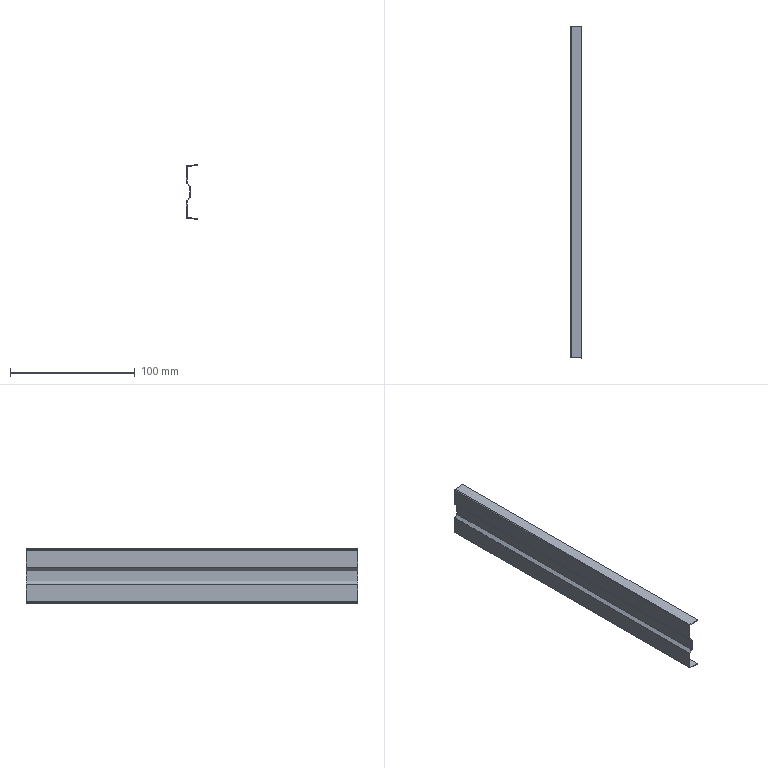Part | NX | features RETAINER-1_5003_009_C-SRH51Y22 2 | 1 solid | 24 faces | box 8.852 x 266.1 x 43.74 mm | volume 9676 mm3 | plane 18 | cylinder 6 | commonest cylinder face diameters 0.8 x4 1.2 x2
STEP:
#1=CARTESIAN_POINT('',(-207.227,-97.3,-65.352));
#2=VERTEX_POINT('',#1);
#3=CARTESIAN_POINT('',(-198.975,-97.3,-64.63));
#4=VERTEX_POINT('',#3);
#5=CARTESIAN_POINT('',(-207.775,-97.3,-65.4));
#6=DIRECTION('',(0.9962,0.,0.08716));
#7=VECTOR('',#6,1000.);
#8=LINE('',#5,#7);
#9=EDGE_CURVE('',#2,#4,#8,.T.);
#10=ORIENTED_EDGE('',*,*,#9,.F.);
#11=CARTESIAN_POINT('',(-207.227,-363.4,-65.352));
#12=VERTEX_POINT('',#11);
#13=CARTESIAN_POINT('',(-207.227,-97.3,-65.352));
#14=DIRECTION('',(0.,-1.,0.));
#15=VECTOR('',#14,1000.);
#16=LINE('',#13,#15);
#17=EDGE_CURVE('',#2,#12,#16,.T.);
#18=ORIENTED_EDGE('',*,*,#17,.T.);
#19=CARTESIAN_POINT('',(-198.975,-363.4,-64.63));
#20=VERTEX_POINT('',#19);
#21=CARTESIAN_POINT('',(-207.775,-363.4,-65.4));
#22=DIRECTION('',(0.9962,0.,0.08716));
#23=VECTOR('',#22,1000.);
#24=LINE('',#21,#23);
#25=EDGE_CURVE('',#12,#20,#24,.T.);
#26=ORIENTED_EDGE('',*,*,#25,.T.);
#27=CARTESIAN_POINT('',(-198.975,-97.3,-64.63));
#28=DIRECTION('',(0.,-1.,0.));
#29=VECTOR('',#28,1000.);
#30=LINE('',#27,#29);
#31=EDGE_CURVE('',#4,#20,#30,.T.);
#32=ORIENTED_EDGE('',*,*,#31,.F.);
#33=EDGE_LOOP('',(#10,#18,#26,#32));
#34=FACE_BOUND('',#33,.T.);
#35=CARTESIAN_POINT('',(-207.775,-97.3,-65.4));
#36=DIRECTION('',(0.08716,0.,-0.9962));
#37=DIRECTION('',(-0.9962,0.,-0.08716));
#38=AXIS2_PLACEMENT_3D('',#35,#36,#37);
#39=PLANE('',#38);
#40=ADVANCED_FACE('',(#34),#39,.F.);
#41=CARTESIAN_POINT('',(-198.923,-363.4,-65.228));
#42=VERTEX_POINT('',#41);
#43=CARTESIAN_POINT('',(-198.975,-363.4,-64.63));
#44=DIRECTION('',(0.08716,0.,-0.9962));
#45=VECTOR('',#44,1000.);
#46=LINE('',#43,#45);
#47=EDGE_CURVE('',#20,#42,#46,.T.);
#48=ORIENTED_EDGE('',*,*,#47,.T.);
#49=CARTESIAN_POINT('',(-198.923,-97.3,-65.228));
#50=VERTEX_POINT('',#49);
#51=CARTESIAN_POINT('',(-198.923,-97.3,-65.228));
#52=DIRECTION('',(0.,-1.,0.));
#53=VECTOR('',#52,1000.);
#54=LINE('',#51,#53);
#55=EDGE_CURVE('',#50,#42,#54,.T.);
#56=ORIENTED_EDGE('',*,*,#55,.F.);
#57=CARTESIAN_POINT('',(-198.975,-97.3,-64.63));
#58=DIRECTION('',(0.08716,0.,-0.9962));
#59=VECTOR('',#58,1000.);
#60=LINE('',#57,#59);
#61=EDGE_CURVE('',#4,#50,#60,.T.);
#62=ORIENTED_EDGE('',*,*,#61,.F.);
#63=ORIENTED_EDGE('',*,*,#31,.T.);
#64=EDGE_LOOP('',(#48,#56,#62,#63));
#65=FACE_BOUND('',#64,.T.);
#66=CARTESIAN_POINT('',(-198.975,-97.3,-64.63));
#67=DIRECTION('',(-0.9962,0.,-0.08716));
#68=DIRECTION('',(-0.08716,0.,0.9962));
#69=AXIS2_PLACEMENT_3D('',#66,#67,#68);
#70=PLANE('',#69);
#71=ADVANCED_FACE('',(#65),#70,.F.);
#72=CARTESIAN_POINT('',(-207.175,-363.4,-65.95));
#73=VERTEX_POINT('',#72);
#74=CARTESIAN_POINT('',(-207.175,-363.4,-65.95));
#75=DIRECTION('',(-0.9962,0.,-0.08716));
#76=VECTOR('',#75,1000.);
#77=LINE('',#74,#76);
#78=EDGE_CURVE('',#42,#73,#77,.T.);
#79=ORIENTED_EDGE('',*,*,#78,.T.);
#80=CARTESIAN_POINT('',(-207.175,-97.3,-65.95));
#81=VERTEX_POINT('',#80);
#82=CARTESIAN_POINT('',(-207.175,-97.3,-65.95));
#83=DIRECTION('',(0.,-1.,0.));
#84=VECTOR('',#83,1000.);
#85=LINE('',#82,#84);
#86=EDGE_CURVE('',#81,#73,#85,.T.);
#87=ORIENTED_EDGE('',*,*,#86,.F.);
#88=CARTESIAN_POINT('',(-207.175,-97.3,-65.95));
#89=DIRECTION('',(-0.9962,0.,-0.08716));
#90=VECTOR('',#89,1000.);
#91=LINE('',#88,#90);
#92=EDGE_CURVE('',#50,#81,#91,.T.);
#93=ORIENTED_EDGE('',*,*,#92,.F.);
#94=ORIENTED_EDGE('',*,*,#55,.T.);
#95=EDGE_LOOP('',(#79,#87,#93,#94));
#96=FACE_BOUND('',#95,.T.);
#97=CARTESIAN_POINT('',(-207.175,-97.3,-65.95));
#98=DIRECTION('',(-0.08716,0.,0.9962));
#99=DIRECTION('',(0.9962,0.,0.08716));
#100=AXIS2_PLACEMENT_3D('',#97,#98,#99);
#101=PLANE('',#100);
#102=ADVANCED_FACE('',(#96),#101,.F.);
#103=CARTESIAN_POINT('',(-207.175,-363.4,-79.4));
#104=VERTEX_POINT('',#103);
#105=CARTESIAN_POINT('',(-207.175,-363.4,-65.95));
#106=DIRECTION('',(0.,0.,-1.));
#107=VECTOR('',#106,1000.);
#108=LINE('',#105,#107);
#109=EDGE_CURVE('',#73,#104,#108,.T.);
#110=ORIENTED_EDGE('',*,*,#109,.T.);
#111=CARTESIAN_POINT('',(-207.175,-97.3,-79.4));
#112=VERTEX_POINT('',#111);
#113=CARTESIAN_POINT('',(-207.175,-97.3,-79.4));
#114=DIRECTION('',(0.,-1.,0.));
#115=VECTOR('',#114,1000.);
#116=LINE('',#113,#115);
#117=EDGE_CURVE('',#112,#104,#116,.T.);
#118=ORIENTED_EDGE('',*,*,#117,.F.);
#119=CARTESIAN_POINT('',(-207.175,-97.3,-65.95));
#120=DIRECTION('',(0.,0.,-1.));
#121=VECTOR('',#120,1000.);
#122=LINE('',#119,#121);
#123=EDGE_CURVE('',#81,#112,#122,.T.);
#124=ORIENTED_EDGE('',*,*,#123,.F.);
#125=ORIENTED_EDGE('',*,*,#86,.T.);
#126=EDGE_LOOP('',(#110,#118,#124,#125));
#127=FACE_BOUND('',#126,.T.);
#128=CARTESIAN_POINT('',(-207.175,-97.3,-65.95));
#129=DIRECTION('',(-1.,0.,0.));
#130=DIRECTION('',(0.,-1.,0.));
#131=AXIS2_PLACEMENT_3D('',#128,#129,#130);
#132=PLANE('',#131);
#133=ADVANCED_FACE('',(#127),#132,.F.);
#134=CARTESIAN_POINT('',(-204.792,-363.4,-81.783));
#135=VERTEX_POINT('',#134);
#136=CARTESIAN_POINT('',(-204.675,-363.4,-81.9));
#137=DIRECTION('',(0.7071,0.,-0.7071));
#138=VECTOR('',#137,1000.);
#139=LINE('',#136,#138);
#140=EDGE_CURVE('',#104,#135,#139,.T.);
#141=ORIENTED_EDGE('',*,*,#140,.T.);
#142=CARTESIAN_POINT('',(-204.792,-97.3,-81.783));
#143=VERTEX_POINT('',#142);
#144=CARTESIAN_POINT('',(-204.792,-97.3,-81.783));
#145=DIRECTION('',(0.,-1.,0.));
#146=VECTOR('',#145,1000.);
#147=LINE('',#144,#146);
#148=EDGE_CURVE('',#135,#143,#147,.F.);
#149=ORIENTED_EDGE('',*,*,#148,.T.);
#150=CARTESIAN_POINT('',(-204.675,-97.3,-81.9));
#151=DIRECTION('',(0.7071,0.,-0.7071));
#152=VECTOR('',#151,1000.);
#153=LINE('',#150,#152);
#154=EDGE_CURVE('',#112,#143,#153,.T.);
#155=ORIENTED_EDGE('',*,*,#154,.F.);
#156=ORIENTED_EDGE('',*,*,#117,.T.);
#157=EDGE_LOOP('',(#141,#149,#155,#156));
#158=FACE_BOUND('',#157,.T.);
#159=CARTESIAN_POINT('',(-204.675,-97.3,-81.9));
#160=DIRECTION('',(-0.7071,0.,-0.7071));
#161=DIRECTION('',(-0.7071,0.,0.7071));
#162=AXIS2_PLACEMENT_3D('',#159,#160,#161);
#163=PLANE('',#162);
#164=ADVANCED_FACE('',(#158),#163,.F.);
#165=CARTESIAN_POINT('',(-204.675,-363.4,-82.066));
#166=VERTEX_POINT('',#165);
#167=CARTESIAN_POINT('',(-204.675,-363.4,-90.934));
#168=VERTEX_POINT('',#167);
#169=CARTESIAN_POINT('',(-204.675,-363.4,-91.1));
#170=DIRECTION('',(0.,0.,-1.));
#171=VECTOR('',#170,1000.);
#172=LINE('',#169,#171);
#173=EDGE_CURVE('',#166,#168,#172,.T.);
#174=ORIENTED_EDGE('',*,*,#173,.T.);
#175=CARTESIAN_POINT('',(-204.675,-97.3,-90.934));
#176=VERTEX_POINT('',#175);
#177=CARTESIAN_POINT('',(-204.675,-97.3,-90.934));
#178=DIRECTION('',(0.,-1.,0.));
#179=VECTOR('',#178,1000.);
#180=LINE('',#177,#179);
#181=EDGE_CURVE('',#168,#176,#180,.F.);
#182=ORIENTED_EDGE('',*,*,#181,.T.);
#183=CARTESIAN_POINT('',(-204.675,-97.3,-82.066));
#184=VERTEX_POINT('',#183);
#185=CARTESIAN_POINT('',(-204.675,-97.3,-91.1));
#186=DIRECTION('',(0.,0.,-1.));
#187=VECTOR('',#186,1000.);
#188=LINE('',#185,#187);
#189=EDGE_CURVE('',#184,#176,#188,.T.);
#190=ORIENTED_EDGE('',*,*,#189,.F.);
#191=CARTESIAN_POINT('',(-204.675,-97.3,-82.066));
#192=DIRECTION('',(0.,-1.,0.));
#193=VECTOR('',#192,1000.);
#194=LINE('',#191,#193);
#195=EDGE_CURVE('',#184,#166,#194,.T.);
#196=ORIENTED_EDGE('',*,*,#195,.T.);
#197=EDGE_LOOP('',(#174,#182,#190,#196));
#198=FACE_BOUND('',#197,.T.);
#199=CARTESIAN_POINT('',(-204.675,-97.3,-91.1));
#200=DIRECTION('',(-1.,0.,0.));
#201=DIRECTION('',(0.,-1.,0.));
#202=AXIS2_PLACEMENT_3D('',#199,#200,#201);
#203=PLANE('',#202);
#204=ADVANCED_FACE('',(#198),#203,.F.);
#205=CARTESIAN_POINT('',(-204.792,-97.3,-91.217));
#206=VERTEX_POINT('',#205);
#207=CARTESIAN_POINT('',(-207.175,-97.3,-93.6));
#208=VERTEX_POINT('',#207);
#209=CARTESIAN_POINT('',(-204.675,-97.3,-91.1));
#210=DIRECTION('',(-0.7071,0.,-0.7071));
#211=VECTOR('',#210,1000.);
#212=LINE('',#209,#211);
#213=EDGE_CURVE('',#206,#208,#212,.T.);
#214=ORIENTED_EDGE('',*,*,#213,.F.);
#215=CARTESIAN_POINT('',(-204.792,-363.4,-91.217));
#216=VERTEX_POINT('',#215);
#217=CARTESIAN_POINT('',(-204.792,-97.3,-91.217));
#218=DIRECTION('',(0.,-1.,0.));
#219=VECTOR('',#218,1000.);
#220=LINE('',#217,#219);
#221=EDGE_CURVE('',#206,#216,#220,.T.);
#222=ORIENTED_EDGE('',*,*,#221,.T.);
#223=CARTESIAN_POINT('',(-207.175,-363.4,-93.6));
#224=VERTEX_POINT('',#223);
#225=CARTESIAN_POINT('',(-204.675,-363.4,-91.1));
#226=DIRECTION('',(-0.7071,0.,-0.7071));
#227=VECTOR('',#226,1000.);
#228=LINE('',#225,#227);
#229=EDGE_CURVE('',#216,#224,#228,.T.);
#230=ORIENTED_EDGE('',*,*,#229,.T.);
#231=CARTESIAN_POINT('',(-207.175,-97.3,-93.6));
#232=DIRECTION('',(0.,-1.,0.));
#233=VECTOR('',#232,1000.);
#234=LINE('',#231,#233);
#235=EDGE_CURVE('',#208,#224,#234,.T.);
#236=ORIENTED_EDGE('',*,*,#235,.F.);
#237=EDGE_LOOP('',(#214,#222,#230,#236));
#238=FACE_BOUND('',#237,.T.);
#239=CARTESIAN_POINT('',(-204.675,-97.3,-91.1));
#240=DIRECTION('',(-0.7071,0.,0.7071));
#241=DIRECTION('',(0.7071,0.,0.7071));
#242=AXIS2_PLACEMENT_3D('',#239,#240,#241);
#243=PLANE('',#242);
#244=ADVANCED_FACE('',(#238),#243,.F.);
#245=CARTESIAN_POINT('',(-207.175,-363.4,-107.05));
#246=VERTEX_POINT('',#245);
#247=CARTESIAN_POINT('',(-207.175,-363.4,-107.05));
#248=DIRECTION('',(0.,0.,-1.));
#249=VECTOR('',#248,1000.);
#250=LINE('',#247,#249);
#251=EDGE_CURVE('',#224,#246,#250,.T.);
#252=ORIENTED_EDGE('',*,*,#251,.T.);
#253=CARTESIAN_POINT('',(-207.175,-97.3,-107.05));
#254=VERTEX_POINT('',#253);
#255=CARTESIAN_POINT('',(-207.175,-97.3,-107.05));
#256=DIRECTION('',(0.,-1.,0.));
#257=VECTOR('',#256,1000.);
#258=LINE('',#255,#257);
#259=EDGE_CURVE('',#254,#246,#258,.T.);
#260=ORIENTED_EDGE('',*,*,#259,.F.);
#261=CARTESIAN_POINT('',(-207.175,-97.3,-107.05));
#262=DIRECTION('',(0.,0.,-1.));
#263=VECTOR('',#262,1000.);
#264=LINE('',#261,#263);
#265=EDGE_CURVE('',#208,#254,#264,.T.);
#266=ORIENTED_EDGE('',*,*,#265,.F.);
#267=ORIENTED_EDGE('',*,*,#235,.T.);
#268=EDGE_LOOP('',(#252,#260,#266,#267));
#269=FACE_BOUND('',#268,.T.);
#270=CARTESIAN_POINT('',(-207.175,-97.3,-107.05));
#271=DIRECTION('',(-1.,0.,0.));
#272=DIRECTION('',(0.,-1.,0.));
#273=AXIS2_PLACEMENT_3D('',#270,#271,#272);
#274=PLANE('',#273);
#275=ADVANCED_FACE('',(#269),#274,.F.);
#276=CARTESIAN_POINT('',(-198.923,-363.4,-107.772));
#277=VERTEX_POINT('',#276);
#278=CARTESIAN_POINT('',(-207.175,-363.4,-107.05));
#279=DIRECTION('',(0.9962,0.,-0.08716));
#280=VECTOR('',#279,1000.);
#281=LINE('',#278,#280);
#282=EDGE_CURVE('',#246,#277,#281,.T.);
#283=ORIENTED_EDGE('',*,*,#282,.T.);
#284=CARTESIAN_POINT('',(-198.923,-97.3,-107.772));
#285=VERTEX_POINT('',#284);
#286=CARTESIAN_POINT('',(-198.923,-97.3,-107.772));
#287=DIRECTION('',(0.,-1.,0.));
#288=VECTOR('',#287,1000.);
#289=LINE('',#286,#288);
#290=EDGE_CURVE('',#285,#277,#289,.T.);
#291=ORIENTED_EDGE('',*,*,#290,.F.);
#292=CARTESIAN_POINT('',(-207.175,-97.3,-107.05));
#293=DIRECTION('',(0.9962,0.,-0.08716));
#294=VECTOR('',#293,1000.);
#295=LINE('',#292,#294);
#296=EDGE_CURVE('',#254,#285,#295,.T.);
#297=ORIENTED_EDGE('',*,*,#296,.F.);
#298=ORIENTED_EDGE('',*,*,#259,.T.);
#299=EDGE_LOOP('',(#283,#291,#297,#298));
#300=FACE_BOUND('',#299,.T.);
#301=CARTESIAN_POINT('',(-207.175,-97.3,-107.05));
#302=DIRECTION('',(-0.08716,0.,-0.9962));
#303=DIRECTION('',(-0.9962,0.,0.08716));
#304=AXIS2_PLACEMENT_3D('',#301,#302,#303);
#305=PLANE('',#304);
#306=ADVANCED_FACE('',(#300),#305,.F.);
#307=CARTESIAN_POINT('',(-198.975,-363.4,-108.37));
#308=VERTEX_POINT('',#307);
#309=CARTESIAN_POINT('',(-198.923,-363.4,-107.772));
#310=DIRECTION('',(-0.08716,0.,-0.9962));
#311=VECTOR('',#310,1000.);
#312=LINE('',#309,#311);
#313=EDGE_CURVE('',#277,#308,#312,.T.);
#314=ORIENTED_EDGE('',*,*,#313,.T.);
#315=CARTESIAN_POINT('',(-198.975,-97.3,-108.37));
#316=VERTEX_POINT('',#315);
#317=CARTESIAN_POINT('',(-198.975,-97.3,-108.37));
#318=DIRECTION('',(0.,-1.,0.));
#319=VECTOR('',#318,1000.);
#320=LINE('',#317,#319);
#321=EDGE_CURVE('',#316,#308,#320,.T.);
#322=ORIENTED_EDGE('',*,*,#321,.F.);
#323=CARTESIAN_POINT('',(-198.923,-97.3,-107.772));
#324=DIRECTION('',(-0.08716,0.,-0.9962));
#325=VECTOR('',#324,1000.);
#326=LINE('',#323,#325);
#327=EDGE_CURVE('',#285,#316,#326,.T.);
#328=ORIENTED_EDGE('',*,*,#327,.F.);
#329=ORIENTED_EDGE('',*,*,#290,.T.);
#330=EDGE_LOOP('',(#314,#322,#328,#329));
#331=FACE_BOUND('',#330,.T.);
#332=CARTESIAN_POINT('',(-198.923,-97.3,-107.772));
#333=DIRECTION('',(-0.9962,0.,0.08716));
#334=DIRECTION('',(0.08716,0.,0.9962));
#335=AXIS2_PLACEMENT_3D('',#332,#333,#334);
#336=PLANE('',#335);
#337=ADVANCED_FACE('',(#331),#336,.F.);
#338=CARTESIAN_POINT('',(-207.227,-363.4,-107.648));
#339=VERTEX_POINT('',#338);
#340=CARTESIAN_POINT('',(-207.775,-363.4,-107.6));
#341=DIRECTION('',(-0.9962,0.,0.08716));
#342=VECTOR('',#341,1000.);
#343=LINE('',#340,#342);
#344=EDGE_CURVE('',#308,#339,#343,.T.);
#345=ORIENTED_EDGE('',*,*,#344,.T.);
#346=CARTESIAN_POINT('',(-207.227,-97.3,-107.648));
#347=VERTEX_POINT('',#346);
#348=CARTESIAN_POINT('',(-207.227,-97.3,-107.648));
#349=DIRECTION('',(0.,-1.,0.));
#350=VECTOR('',#349,1000.);
#351=LINE('',#348,#350);
#352=EDGE_CURVE('',#339,#347,#351,.F.);
#353=ORIENTED_EDGE('',*,*,#352,.T.);
#354=CARTESIAN_POINT('',(-207.775,-97.3,-107.6));
#355=DIRECTION('',(-0.9962,0.,0.08716));
#356=VECTOR('',#355,1000.);
#357=LINE('',#354,#356);
#358=EDGE_CURVE('',#316,#347,#357,.T.);
#359=ORIENTED_EDGE('',*,*,#358,.F.);
#360=ORIENTED_EDGE('',*,*,#321,.T.);
#361=EDGE_LOOP('',(#345,#353,#359,#360));
#362=FACE_BOUND('',#361,.T.);
#363=CARTESIAN_POINT('',(-207.775,-97.3,-107.6));
#364=DIRECTION('',(0.08716,0.,0.9962));
#365=DIRECTION('',(0.9962,0.,-0.08716));
#366=AXIS2_PLACEMENT_3D('',#363,#364,#365);
#367=PLANE('',#366);
#368=ADVANCED_FACE('',(#362),#367,.F.);
#369=CARTESIAN_POINT('',(-207.775,-363.4,-107.05));
#370=VERTEX_POINT('',#369);
#371=CARTESIAN_POINT('',(-207.775,-363.4,-93.517));
#372=VERTEX_POINT('',#371);
#373=CARTESIAN_POINT('',(-207.775,-363.4,-107.6));
#374=DIRECTION('',(0.,0.,1.));
#375=VECTOR('',#374,1000.);
#376=LINE('',#373,#375);
#377=EDGE_CURVE('',#370,#372,#376,.T.);
#378=ORIENTED_EDGE('',*,*,#377,.T.);
#379=CARTESIAN_POINT('',(-207.775,-97.3,-93.517));
#380=VERTEX_POINT('',#379);
#381=CARTESIAN_POINT('',(-207.775,-97.3,-93.517));
#382=DIRECTION('',(0.,-1.,0.));
#383=VECTOR('',#382,1000.);
#384=LINE('',#381,#383);
#385=EDGE_CURVE('',#372,#380,#384,.F.);
#386=ORIENTED_EDGE('',*,*,#385,.T.);
#387=CARTESIAN_POINT('',(-207.775,-97.3,-107.05));
#388=VERTEX_POINT('',#387);
#389=CARTESIAN_POINT('',(-207.775,-97.3,-107.6));
#390=DIRECTION('',(0.,0.,1.));
#391=VECTOR('',#390,1000.);
#392=LINE('',#389,#391);
#393=EDGE_CURVE('',#388,#380,#392,.T.);
#394=ORIENTED_EDGE('',*,*,#393,.F.);
#395=CARTESIAN_POINT('',(-207.775,-97.3,-107.05));
#396=DIRECTION('',(0.,-1.,0.));
#397=VECTOR('',#396,1000.);
#398=LINE('',#395,#397);
#399=EDGE_CURVE('',#388,#370,#398,.T.);
#400=ORIENTED_EDGE('',*,*,#399,.T.);
#401=EDGE_LOOP('',(#378,#386,#394,#400));
#402=FACE_BOUND('',#401,.T.);
#403=CARTESIAN_POINT('',(-207.775,-97.3,-107.6));
#404=DIRECTION('',(1.,0.,0.));
#405=DIRECTION('',(0.,0.,-1.));
#406=AXIS2_PLACEMENT_3D('',#403,#404,#405);
#407=PLANE('',#406);
#408=ADVANCED_FACE('',(#402),#407,.F.);
#409=CARTESIAN_POINT('',(-207.658,-97.3,-93.234));
#410=VERTEX_POINT('',#409);
#411=CARTESIAN_POINT('',(-205.275,-97.3,-90.851));
#412=VERTEX_POINT('',#411);
#413=CARTESIAN_POINT('',(-205.275,-97.3,-90.851));
#414=DIRECTION('',(0.7071,0.,0.7071));
#415=VECTOR('',#414,1000.);
#416=LINE('',#413,#415);
#417=EDGE_CURVE('',#410,#412,#416,.T.);
#418=ORIENTED_EDGE('',*,*,#417,.F.);
#419=CARTESIAN_POINT('',(-207.658,-363.4,-93.234));
#420=VERTEX_POINT('',#419);
#421=CARTESIAN_POINT('',(-207.658,-97.3,-93.234));
#422=DIRECTION('',(0.,-1.,0.));
#423=VECTOR('',#422,1000.);
#424=LINE('',#421,#423);
#425=EDGE_CURVE('',#410,#420,#424,.T.);
#426=ORIENTED_EDGE('',*,*,#425,.T.);
#427=CARTESIAN_POINT('',(-205.275,-363.4,-90.851));
#428=VERTEX_POINT('',#427);
#429=CARTESIAN_POINT('',(-205.275,-363.4,-90.851));
#430=DIRECTION('',(0.7071,0.,0.7071));
#431=VECTOR('',#430,1000.);
#432=LINE('',#429,#431);
#433=EDGE_CURVE('',#420,#428,#432,.T.);
#434=ORIENTED_EDGE('',*,*,#433,.T.);
#435=CARTESIAN_POINT('',(-205.275,-97.3,-90.851));
#436=DIRECTION('',(0.,-1.,0.));
#437=VECTOR('',#436,1000.);
#438=LINE('',#435,#437);
#439=EDGE_CURVE('',#412,#428,#438,.T.);
#440=ORIENTED_EDGE('',*,*,#439,.F.);
#441=EDGE_LOOP('',(#418,#426,#434,#440));
#442=FACE_BOUND('',#441,.T.);
#443=CARTESIAN_POINT('',(-205.275,-97.3,-90.851));
#444=DIRECTION('',(0.7071,0.,-0.7071));
#445=DIRECTION('',(-0.7071,0.,-0.7071));
#446=AXIS2_PLACEMENT_3D('',#443,#444,#445);
#447=PLANE('',#446);
#448=ADVANCED_FACE('',(#442),#447,.F.);
#449=CARTESIAN_POINT('',(-205.275,-363.4,-82.149));
#450=VERTEX_POINT('',#449);
#451=CARTESIAN_POINT('',(-205.275,-363.4,-90.851));
#452=DIRECTION('',(0.,0.,1.));
#453=VECTOR('',#452,1000.);
#454=LINE('',#451,#453);
#455=EDGE_CURVE('',#428,#450,#454,.T.);
#456=ORIENTED_EDGE('',*,*,#455,.T.);
#457=CARTESIAN_POINT('',(-205.275,-97.3,-82.149));
#458=VERTEX_POINT('',#457);
#459=CARTESIAN_POINT('',(-205.275,-97.3,-82.149));
#460=DIRECTION('',(0.,-1.,0.));
#461=VECTOR('',#460,1000.);
#462=LINE('',#459,#461);
#463=EDGE_CURVE('',#458,#450,#462,.T.);
#464=ORIENTED_EDGE('',*,*,#463,.F.);
#465=CARTESIAN_POINT('',(-205.275,-97.3,-90.851));
#466=DIRECTION('',(0.,0.,1.));
#467=VECTOR('',#466,1000.);
#468=LINE('',#465,#467);
#469=EDGE_CURVE('',#412,#458,#468,.T.);
#470=ORIENTED_EDGE('',*,*,#469,.F.);
#471=ORIENTED_EDGE('',*,*,#439,.T.);
#472=EDGE_LOOP('',(#456,#464,#470,#471));
#473=FACE_BOUND('',#472,.T.);
#474=CARTESIAN_POINT('',(-205.275,-97.3,-90.851));
#475=DIRECTION('',(1.,0.,0.));
#476=DIRECTION('',(0.,1.,0.));
#477=AXIS2_PLACEMENT_3D('',#474,#475,#476);
#478=PLANE('',#477);
#479=ADVANCED_FACE('',(#473),#478,.F.);
#480=CARTESIAN_POINT('',(-207.658,-363.4,-79.766));
#481=VERTEX_POINT('',#480);
#482=CARTESIAN_POINT('',(-205.275,-363.4,-82.149));
#483=DIRECTION('',(-0.7071,0.,0.7071));
#484=VECTOR('',#483,1000.);
#485=LINE('',#482,#484);
#486=EDGE_CURVE('',#450,#481,#485,.T.);
#487=ORIENTED_EDGE('',*,*,#486,.T.);
#488=CARTESIAN_POINT('',(-207.658,-97.3,-79.766));
#489=VERTEX_POINT('',#488);
#490=CARTESIAN_POINT('',(-207.658,-97.3,-79.766));
#491=DIRECTION('',(0.,-1.,0.));
#492=VECTOR('',#491,1000.);
#493=LINE('',#490,#492);
#494=EDGE_CURVE('',#481,#489,#493,.F.);
#495=ORIENTED_EDGE('',*,*,#494,.T.);
#496=CARTESIAN_POINT('',(-205.275,-97.3,-82.149));
#497=DIRECTION('',(-0.7071,0.,0.7071));
#498=VECTOR('',#497,1000.);
#499=LINE('',#496,#498);
#500=EDGE_CURVE('',#458,#489,#499,.T.);
#501=ORIENTED_EDGE('',*,*,#500,.F.);
#502=ORIENTED_EDGE('',*,*,#463,.T.);
#503=EDGE_LOOP('',(#487,#495,#501,#502));
#504=FACE_BOUND('',#503,.T.);
#505=CARTESIAN_POINT('',(-205.275,-97.3,-82.149));
#506=DIRECTION('',(0.7071,0.,0.7071));
#507=DIRECTION('',(0.7071,0.,-0.7071));
#508=AXIS2_PLACEMENT_3D('',#505,#506,#507);
#509=PLANE('',#508);
#510=ADVANCED_FACE('',(#504),#509,.F.);
#511=CARTESIAN_POINT('',(-207.775,-97.3,-79.483));
#512=VERTEX_POINT('',#511);
#513=CARTESIAN_POINT('',(-207.775,-97.3,-65.95));
#514=VERTEX_POINT('',#513);
#515=CARTESIAN_POINT('',(-207.775,-97.3,-65.4));
#516=DIRECTION('',(0.,0.,1.));
#517=VECTOR('',#516,1000.);
#518=LINE('',#515,#517);
#519=EDGE_CURVE('',#512,#514,#518,.T.);
#520=ORIENTED_EDGE('',*,*,#519,.F.);
#521=CARTESIAN_POINT('',(-207.775,-363.4,-79.483));
#522=VERTEX_POINT('',#521);
#523=CARTESIAN_POINT('',(-207.775,-97.3,-79.483));
#524=DIRECTION('',(0.,-1.,0.));
#525=VECTOR('',#524,1000.);
#526=LINE('',#523,#525);
#527=EDGE_CURVE('',#512,#522,#526,.T.);
#528=ORIENTED_EDGE('',*,*,#527,.T.);
#529=CARTESIAN_POINT('',(-207.775,-363.4,-65.95));
#530=VERTEX_POINT('',#529);
#531=CARTESIAN_POINT('',(-207.775,-363.4,-65.4));
#532=DIRECTION('',(0.,0.,1.));
#533=VECTOR('',#532,1000.);
#534=LINE('',#531,#533);
#535=EDGE_CURVE('',#522,#530,#534,.T.);
#536=ORIENTED_EDGE('',*,*,#535,.T.);
#537=CARTESIAN_POINT('',(-207.775,-97.3,-65.95));
#538=DIRECTION('',(0.,-1.,0.));
#539=VECTOR('',#538,1000.);
#540=LINE('',#537,#539);
#541=EDGE_CURVE('',#530,#514,#540,.F.);
#542=ORIENTED_EDGE('',*,*,#541,.T.);
#543=EDGE_LOOP('',(#520,#528,#536,#542));
#544=FACE_BOUND('',#543,.T.);
#545=CARTESIAN_POINT('',(-207.775,-97.3,-65.4));
#546=DIRECTION('',(1.,0.,0.));
#547=DIRECTION('',(0.,0.,-1.));
#548=AXIS2_PLACEMENT_3D('',#545,#546,#547);
#549=PLANE('',#548);
#550=ADVANCED_FACE('',(#544),#549,.F.);
#551=ORIENTED_EDGE('',*,*,#189,.T.);
#552=CARTESIAN_POINT('',(-205.075,-97.3,-90.934));
#553=DIRECTION('',(0.,1.,0.));
#554=DIRECTION('',(-1.,0.,0.));
#555=AXIS2_PLACEMENT_3D('',#552,#553,#554);
#556=CIRCLE('',#555,0.4);
#557=EDGE_CURVE('',#176,#206,#556,.T.);
#558=ORIENTED_EDGE('',*,*,#557,.T.);
#559=ORIENTED_EDGE('',*,*,#213,.T.);
#560=ORIENTED_EDGE('',*,*,#265,.T.);
#561=ORIENTED_EDGE('',*,*,#296,.T.);
#562=ORIENTED_EDGE('',*,*,#327,.T.);
#563=ORIENTED_EDGE('',*,*,#358,.T.);
#564=CARTESIAN_POINT('',(-207.175,-97.3,-107.05));
#565=DIRECTION('',(0.,1.,0.));
#566=DIRECTION('',(-1.,0.,0.));
#567=AXIS2_PLACEMENT_3D('',#564,#565,#566);
#568=CIRCLE('',#567,0.6);
#569=EDGE_CURVE('',#347,#388,#568,.T.);
#570=ORIENTED_EDGE('',*,*,#569,.T.);
#571=ORIENTED_EDGE('',*,*,#393,.T.);
#572=CARTESIAN_POINT('',(-207.375,-97.3,-93.517));
#573=DIRECTION('',(0.,1.,0.));
#574=DIRECTION('',(-1.,0.,0.));
#575=AXIS2_PLACEMENT_3D('',#572,#573,#574);
#576=CIRCLE('',#575,0.4);
#577=EDGE_CURVE('',#380,#410,#576,.T.);
#578=ORIENTED_EDGE('',*,*,#577,.T.);
#579=ORIENTED_EDGE('',*,*,#417,.T.);
#580=ORIENTED_EDGE('',*,*,#469,.T.);
#581=ORIENTED_EDGE('',*,*,#500,.T.);
#582=CARTESIAN_POINT('',(-207.375,-97.3,-79.483));
#583=DIRECTION('',(0.,1.,0.));
#584=DIRECTION('',(-1.,0.,0.));
#585=AXIS2_PLACEMENT_3D('',#582,#583,#584);
#586=CIRCLE('',#585,0.4);
#587=EDGE_CURVE('',#489,#512,#586,.T.);
#588=ORIENTED_EDGE('',*,*,#587,.T.);
#589=ORIENTED_EDGE('',*,*,#519,.T.);
#590=CARTESIAN_POINT('',(-207.175,-97.3,-65.95));
#591=DIRECTION('',(0.,1.,0.));
#592=DIRECTION('',(-1.,0.,0.));
#593=AXIS2_PLACEMENT_3D('',#590,#591,#592);
#594=CIRCLE('',#593,0.6);
#595=EDGE_CURVE('',#514,#2,#594,.T.);
#596=ORIENTED_EDGE('',*,*,#595,.T.);
#597=ORIENTED_EDGE('',*,*,#9,.T.);
#598=ORIENTED_EDGE('',*,*,#61,.T.);
#599=ORIENTED_EDGE('',*,*,#92,.T.);
#600=ORIENTED_EDGE('',*,*,#123,.T.);
#601=ORIENTED_EDGE('',*,*,#154,.T.);
#602=CARTESIAN_POINT('',(-205.075,-97.3,-82.066));
#603=DIRECTION('',(0.,1.,0.));
#604=DIRECTION('',(-1.,0.,0.));
#605=AXIS2_PLACEMENT_3D('',#602,#603,#604);
#606=CIRCLE('',#605,0.4);
#607=EDGE_CURVE('',#143,#184,#606,.T.);
#608=ORIENTED_EDGE('',*,*,#607,.T.);
#609=EDGE_LOOP('',(#551,#558,#559,#560,#561,#562,#563,#570,#571,#578,#579,#580,#581,#588,#589,#596,#597,#598,#599,#600,#601,#608));
#610=FACE_BOUND('',#609,.T.);
#611=CARTESIAN_POINT('',(-202.275,-97.3,-86.5));
#612=DIRECTION('',(0.,1.,0.));
#613=DIRECTION('',(-1.,0.,0.));
#614=AXIS2_PLACEMENT_3D('',#611,#612,#613);
#615=PLANE('',#614);
#616=ADVANCED_FACE('',(#610),#615,.T.);
#617=ORIENTED_EDGE('',*,*,#229,.F.);
#618=CARTESIAN_POINT('',(-205.075,-363.4,-90.934));
#619=DIRECTION('',(0.,1.,0.));
#620=DIRECTION('',(-1.,0.,0.));
#621=AXIS2_PLACEMENT_3D('',#618,#619,#620);
#622=CIRCLE('',#621,0.4);
#623=EDGE_CURVE('',#216,#168,#622,.F.);
#624=ORIENTED_EDGE('',*,*,#623,.T.);
#625=ORIENTED_EDGE('',*,*,#173,.F.);
#626=CARTESIAN_POINT('',(-205.075,-363.4,-82.066));
#627=DIRECTION('',(0.,1.,0.));
#628=DIRECTION('',(-1.,0.,0.));
#629=AXIS2_PLACEMENT_3D('',#626,#627,#628);
#630=CIRCLE('',#629,0.4);
#631=EDGE_CURVE('',#166,#135,#630,.F.);
#632=ORIENTED_EDGE('',*,*,#631,.T.);
#633=ORIENTED_EDGE('',*,*,#140,.F.);
#634=ORIENTED_EDGE('',*,*,#109,.F.);
#635=ORIENTED_EDGE('',*,*,#78,.F.);
#636=ORIENTED_EDGE('',*,*,#47,.F.);
#637=ORIENTED_EDGE('',*,*,#25,.F.);
#638=CARTESIAN_POINT('',(-207.175,-363.4,-65.95));
#639=DIRECTION('',(0.,1.,0.));
#640=DIRECTION('',(-1.,0.,0.));
#641=AXIS2_PLACEMENT_3D('',#638,#639,#640);
#642=CIRCLE('',#641,0.6);
#643=EDGE_CURVE('',#12,#530,#642,.F.);
#644=ORIENTED_EDGE('',*,*,#643,.T.);
#645=ORIENTED_EDGE('',*,*,#535,.F.);
#646=CARTESIAN_POINT('',(-207.375,-363.4,-79.483));
#647=DIRECTION('',(0.,1.,0.));
#648=DIRECTION('',(-1.,0.,0.));
#649=AXIS2_PLACEMENT_3D('',#646,#647,#648);
#650=CIRCLE('',#649,0.4);
#651=EDGE_CURVE('',#522,#481,#650,.F.);
#652=ORIENTED_EDGE('',*,*,#651,.T.);
#653=ORIENTED_EDGE('',*,*,#486,.F.);
#654=ORIENTED_EDGE('',*,*,#455,.F.);
#655=ORIENTED_EDGE('',*,*,#433,.F.);
#656=CARTESIAN_POINT('',(-207.375,-363.4,-93.517));
#657=DIRECTION('',(0.,1.,0.));
#658=DIRECTION('',(-1.,0.,0.));
#659=AXIS2_PLACEMENT_3D('',#656,#657,#658);
#660=CIRCLE('',#659,0.4);
#661=EDGE_CURVE('',#420,#372,#660,.F.);
#662=ORIENTED_EDGE('',*,*,#661,.T.);
#663=ORIENTED_EDGE('',*,*,#377,.F.);
#664=CARTESIAN_POINT('',(-207.175,-363.4,-107.05));
#665=DIRECTION('',(0.,1.,0.));
#666=DIRECTION('',(-1.,0.,0.));
#667=AXIS2_PLACEMENT_3D('',#664,#665,#666);
#668=CIRCLE('',#667,0.6);
#669=EDGE_CURVE('',#370,#339,#668,.F.);
#670=ORIENTED_EDGE('',*,*,#669,.T.);
#671=ORIENTED_EDGE('',*,*,#344,.F.);
#672=ORIENTED_EDGE('',*,*,#313,.F.);
#673=ORIENTED_EDGE('',*,*,#282,.F.);
#674=ORIENTED_EDGE('',*,*,#251,.F.);
#675=EDGE_LOOP('',(#617,#624,#625,#632,#633,#634,#635,#636,#637,#644,#645,#652,#653,#654,#655,#662,#663,#670,#671,#672,#673,#674));
#676=FACE_BOUND('',#675,.T.);
#677=CARTESIAN_POINT('',(-202.275,-363.4,-86.5));
#678=DIRECTION('',(0.,1.,0.));
#679=DIRECTION('',(-1.,0.,0.));
#680=AXIS2_PLACEMENT_3D('',#677,#678,#679);
#681=PLANE('',#680);
#682=ADVANCED_FACE('',(#676),#681,.F.);
#683=ORIENTED_EDGE('',*,*,#569,.F.);
#684=ORIENTED_EDGE('',*,*,#352,.F.);
#685=ORIENTED_EDGE('',*,*,#669,.F.);
#686=ORIENTED_EDGE('',*,*,#399,.F.);
#687=EDGE_LOOP('',(#683,#684,#685,#686));
#688=FACE_BOUND('',#687,.T.);
#689=CARTESIAN_POINT('',(-207.175,-97.3,-107.05));
#690=DIRECTION('',(0.,-1.,0.));
#691=DIRECTION('',(1.,0.,0.));
#692=AXIS2_PLACEMENT_3D('',#689,#690,#691);
#693=CYLINDRICAL_SURFACE('',#692,0.6);
#694=ADVANCED_FACE('',(#688),#693,.T.);
#695=ORIENTED_EDGE('',*,*,#595,.F.);
#696=ORIENTED_EDGE('',*,*,#541,.F.);
#697=ORIENTED_EDGE('',*,*,#643,.F.);
#698=ORIENTED_EDGE('',*,*,#17,.F.);
#699=EDGE_LOOP('',(#695,#696,#697,#698));
#700=FACE_BOUND('',#699,.T.);
#701=CARTESIAN_POINT('',(-207.175,-97.3,-65.95));
#702=DIRECTION('',(0.,-1.,0.));
#703=DIRECTION('',(1.,0.,0.));
#704=AXIS2_PLACEMENT_3D('',#701,#702,#703);
#705=CYLINDRICAL_SURFACE('',#704,0.6);
#706=ADVANCED_FACE('',(#700),#705,.T.);
#707=ORIENTED_EDGE('',*,*,#557,.F.);
#708=ORIENTED_EDGE('',*,*,#181,.F.);
#709=ORIENTED_EDGE('',*,*,#623,.F.);
#710=ORIENTED_EDGE('',*,*,#221,.F.);
#711=EDGE_LOOP('',(#707,#708,#709,#710));
#712=FACE_BOUND('',#711,.T.);
#713=CARTESIAN_POINT('',(-205.075,-97.3,-90.934));
#714=DIRECTION('',(0.,-1.,0.));
#715=DIRECTION('',(1.,0.,0.));
#716=AXIS2_PLACEMENT_3D('',#713,#714,#715);
#717=CYLINDRICAL_SURFACE('',#716,0.4);
#718=ADVANCED_FACE('',(#712),#717,.T.);
#719=ORIENTED_EDGE('',*,*,#607,.F.);
#720=ORIENTED_EDGE('',*,*,#148,.F.);
#721=ORIENTED_EDGE('',*,*,#631,.F.);
#722=ORIENTED_EDGE('',*,*,#195,.F.);
#723=EDGE_LOOP('',(#719,#720,#721,#722));
#724=FACE_BOUND('',#723,.T.);
#725=CARTESIAN_POINT('',(-205.075,-97.3,-82.066));
#726=DIRECTION('',(0.,-1.,0.));
#727=DIRECTION('',(1.,0.,0.));
#728=AXIS2_PLACEMENT_3D('',#725,#726,#727);
#729=CYLINDRICAL_SURFACE('',#728,0.4);
#730=ADVANCED_FACE('',(#724),#729,.T.);
#731=ORIENTED_EDGE('',*,*,#577,.F.);
#732=ORIENTED_EDGE('',*,*,#385,.F.);
#733=ORIENTED_EDGE('',*,*,#661,.F.);
#734=ORIENTED_EDGE('',*,*,#425,.F.);
#735=EDGE_LOOP('',(#731,#732,#733,#734));
#736=FACE_BOUND('',#735,.T.);
#737=CARTESIAN_POINT('',(-207.375,-97.3,-93.517));
#738=DIRECTION('',(0.,-1.,0.));
#739=DIRECTION('',(1.,0.,0.));
#740=AXIS2_PLACEMENT_3D('',#737,#738,#739);
#741=CYLINDRICAL_SURFACE('',#740,0.4);
#742=ADVANCED_FACE('',(#736),#741,.T.);
#743=ORIENTED_EDGE('',*,*,#587,.F.);
#744=ORIENTED_EDGE('',*,*,#494,.F.);
#745=ORIENTED_EDGE('',*,*,#651,.F.);
#746=ORIENTED_EDGE('',*,*,#527,.F.);
#747=EDGE_LOOP('',(#743,#744,#745,#746));
#748=FACE_BOUND('',#747,.T.);
#749=CARTESIAN_POINT('',(-207.375,-97.3,-79.483));
#750=DIRECTION('',(0.,-1.,0.));
#751=DIRECTION('',(1.,0.,0.));
#752=AXIS2_PLACEMENT_3D('',#749,#750,#751);
#753=CYLINDRICAL_SURFACE('',#752,0.4);
#754=ADVANCED_FACE('',(#748),#753,.T.);
#755=CLOSED_SHELL('',(#40,#71,#102,#133,#164,#204,#244,#275,#306,#337,#368,#408,#448,#479,#510,#550,#616,#682,#694,#706,#718,#730,#742,#754));
#756=MANIFOLD_SOLID_BREP('',#755);
#757=(LENGTH_UNIT()NAMED_UNIT(*)SI_UNIT(.MILLI.,.METRE.));
#758=UNCERTAINTY_MEASURE_WITH_UNIT(LENGTH_MEASURE(0.00001),#757,'','');
#759=(NAMED_UNIT(*)PLANE_ANGLE_UNIT()SI_UNIT($,.RADIAN.));
#760=(NAMED_UNIT(*)SI_UNIT($,.STERADIAN.)SOLID_ANGLE_UNIT());
#761=(GEOMETRIC_REPRESENTATION_CONTEXT(3)GLOBAL_UNCERTAINTY_ASSIGNED_CONTEXT((#758))GLOBAL_UNIT_ASSIGNED_CONTEXT((#757,#759,#760))REPRESENTATION_CONTEXT('',''));
#762=ADVANCED_BREP_SHAPE_REPRESENTATION('',(#756),#761);